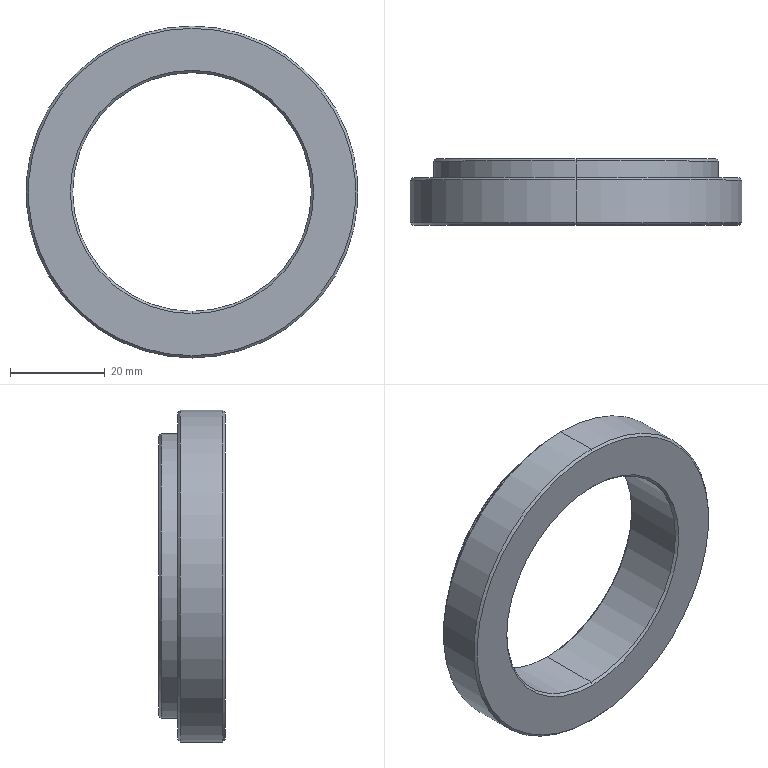Part | STEP file | 10-07 top ring | 1 solid | 19 faces | box 70 x 14 x 70 mm | volume 21857 mm3 | cone 10 | cylinder 6 | plane 3 | commonest cylinder face diameters 50.3 x2 60 x2 70 x2
STEP:
#1=CARTESIAN_POINT('',(0.,3.5,-25.15));
#2=VERTEX_POINT('',#1);
#3=CARTESIAN_POINT('',(0.,3.5,25.15));
#4=VERTEX_POINT('',#3);
#5=CARTESIAN_POINT('',(0.,3.5,0.));
#6=DIRECTION('',(0.,1.,0.));
#7=DIRECTION('',(0.,0.,1.));
#8=AXIS2_PLACEMENT_3D('',#5,#6,#7);
#9=CIRCLE('',#8,25.15);
#10=EDGE_CURVE('',#2,#4,#9,.T.);
#11=ORIENTED_EDGE('',*,*,#10,.F.);
#12=CARTESIAN_POINT('',(0.,4.,-25.65));
#13=VERTEX_POINT('',#12);
#14=CARTESIAN_POINT('',(0.,3.5,-25.15));
#15=DIRECTION('',(0.,0.7071,-0.7071));
#16=VECTOR('',#15,1000.);
#17=LINE('',#14,#16);
#18=EDGE_CURVE('',#2,#13,#17,.T.);
#19=ORIENTED_EDGE('',*,*,#18,.T.);
#20=CARTESIAN_POINT('',(0.,4.,25.65));
#21=VERTEX_POINT('',#20);
#22=CARTESIAN_POINT('',(0.,4.,0.));
#23=DIRECTION('',(0.,-1.,0.));
#24=DIRECTION('',(0.,0.,1.));
#25=AXIS2_PLACEMENT_3D('',#22,#23,#24);
#26=CIRCLE('',#25,25.65);
#27=EDGE_CURVE('',#21,#13,#26,.T.);
#28=ORIENTED_EDGE('',*,*,#27,.F.);
#29=CARTESIAN_POINT('',(0.,3.5,25.15));
#30=DIRECTION('',(0.,0.7071,0.7071));
#31=VECTOR('',#30,1000.);
#32=LINE('',#29,#31);
#33=EDGE_CURVE('',#4,#21,#32,.T.);
#34=ORIENTED_EDGE('',*,*,#33,.F.);
#35=EDGE_LOOP('',(#11,#19,#28,#34));
#36=FACE_OUTER_BOUND('',#35,.T.);
#37=CARTESIAN_POINT('',(0.,3.5,0.));
#38=DIRECTION('',(0.,1.,0.));
#39=DIRECTION('',(0.,0.,1.));
#40=AXIS2_PLACEMENT_3D('',#37,#38,#39);
#41=CONICAL_SURFACE('',#40,25.15,0.7854);
#42=ADVANCED_FACE('',(#36),#41,.F.);
#43=CARTESIAN_POINT('',(0.,4.,29.5));
#44=VERTEX_POINT('',#43);
#45=CARTESIAN_POINT('',(0.,4.,-29.5));
#46=VERTEX_POINT('',#45);
#47=CARTESIAN_POINT('',(0.,4.,0.));
#48=DIRECTION('',(0.,1.,0.));
#49=DIRECTION('',(0.,0.,1.));
#50=AXIS2_PLACEMENT_3D('',#47,#48,#49);
#51=CIRCLE('',#50,29.5);
#52=EDGE_CURVE('',#44,#46,#51,.T.);
#53=ORIENTED_EDGE('',*,*,#52,.F.);
#54=CARTESIAN_POINT('',(0.,3.5,30.));
#55=VERTEX_POINT('',#54);
#56=CARTESIAN_POINT('',(0.,4.,29.5));
#57=DIRECTION('',(0.,-0.7071,0.7071));
#58=VECTOR('',#57,1000.);
#59=LINE('',#56,#58);
#60=EDGE_CURVE('',#44,#55,#59,.T.);
#61=ORIENTED_EDGE('',*,*,#60,.T.);
#62=CARTESIAN_POINT('',(0.,3.5,-30.));
#63=VERTEX_POINT('',#62);
#64=CARTESIAN_POINT('',(0.,3.5,0.));
#65=DIRECTION('',(0.,-1.,0.));
#66=DIRECTION('',(0.,0.,1.));
#67=AXIS2_PLACEMENT_3D('',#64,#65,#66);
#68=CIRCLE('',#67,30.);
#69=EDGE_CURVE('',#63,#55,#68,.T.);
#70=ORIENTED_EDGE('',*,*,#69,.F.);
#71=CARTESIAN_POINT('',(0.,4.,-29.5));
#72=DIRECTION('',(0.,-0.7071,-0.7071));
#73=VECTOR('',#72,1000.);
#74=LINE('',#71,#73);
#75=EDGE_CURVE('',#46,#63,#74,.T.);
#76=ORIENTED_EDGE('',*,*,#75,.F.);
#77=EDGE_LOOP('',(#53,#61,#70,#76));
#78=FACE_OUTER_BOUND('',#77,.T.);
#79=CARTESIAN_POINT('',(0.,4.,0.));
#80=DIRECTION('',(0.,-1.,0.));
#81=DIRECTION('',(0.,0.,-1.));
#82=AXIS2_PLACEMENT_3D('',#79,#80,#81);
#83=CONICAL_SURFACE('',#82,29.5,0.7854);
#84=ADVANCED_FACE('',(#78),#83,.T.);
#85=CARTESIAN_POINT('',(0.,-9.5,25.15));
#86=VERTEX_POINT('',#85);
#87=CARTESIAN_POINT('',(0.,-9.5,-25.15));
#88=VERTEX_POINT('',#87);
#89=CARTESIAN_POINT('',(0.,-9.5,0.));
#90=DIRECTION('',(0.,-1.,0.));
#91=DIRECTION('',(0.,0.,-1.));
#92=AXIS2_PLACEMENT_3D('',#89,#90,#91);
#93=CIRCLE('',#92,25.15);
#94=EDGE_CURVE('',#86,#88,#93,.T.);
#95=ORIENTED_EDGE('',*,*,#94,.F.);
#96=CARTESIAN_POINT('',(0.,-10.,25.65));
#97=VERTEX_POINT('',#96);
#98=CARTESIAN_POINT('',(0.,-9.5,25.15));
#99=DIRECTION('',(0.,-0.7071,0.7071));
#100=VECTOR('',#99,1000.);
#101=LINE('',#98,#100);
#102=EDGE_CURVE('',#86,#97,#101,.T.);
#103=ORIENTED_EDGE('',*,*,#102,.T.);
#104=CARTESIAN_POINT('',(0.,-10.,-25.65));
#105=VERTEX_POINT('',#104);
#106=CARTESIAN_POINT('',(0.,-10.,0.));
#107=DIRECTION('',(0.,1.,0.));
#108=DIRECTION('',(0.,0.,-1.));
#109=AXIS2_PLACEMENT_3D('',#106,#107,#108);
#110=CIRCLE('',#109,25.65);
#111=EDGE_CURVE('',#105,#97,#110,.T.);
#112=ORIENTED_EDGE('',*,*,#111,.F.);
#113=CARTESIAN_POINT('',(0.,-9.5,-25.15));
#114=DIRECTION('',(0.,-0.7071,-0.7071));
#115=VECTOR('',#114,1000.);
#116=LINE('',#113,#115);
#117=EDGE_CURVE('',#88,#105,#116,.T.);
#118=ORIENTED_EDGE('',*,*,#117,.F.);
#119=EDGE_LOOP('',(#95,#103,#112,#118));
#120=FACE_OUTER_BOUND('',#119,.T.);
#121=CARTESIAN_POINT('',(0.,-9.5,0.));
#122=DIRECTION('',(0.,-1.,0.));
#123=DIRECTION('',(0.,0.,-1.));
#124=AXIS2_PLACEMENT_3D('',#121,#122,#123);
#125=CONICAL_SURFACE('',#124,25.15,0.7854);
#126=ADVANCED_FACE('',(#120),#125,.F.);
#127=CARTESIAN_POINT('',(0.,-10.,-34.5));
#128=VERTEX_POINT('',#127);
#129=CARTESIAN_POINT('',(0.,-10.,34.5));
#130=VERTEX_POINT('',#129);
#131=CARTESIAN_POINT('',(0.,-10.,0.));
#132=DIRECTION('',(0.,-1.,0.));
#133=DIRECTION('',(0.,0.,-1.));
#134=AXIS2_PLACEMENT_3D('',#131,#132,#133);
#135=CIRCLE('',#134,34.5);
#136=EDGE_CURVE('',#128,#130,#135,.T.);
#137=ORIENTED_EDGE('',*,*,#136,.F.);
#138=CARTESIAN_POINT('',(0.,-9.5,-35.));
#139=VERTEX_POINT('',#138);
#140=CARTESIAN_POINT('',(0.,-10.,-34.5));
#141=DIRECTION('',(0.,0.7071,-0.7071));
#142=VECTOR('',#141,1000.);
#143=LINE('',#140,#142);
#144=EDGE_CURVE('',#128,#139,#143,.T.);
#145=ORIENTED_EDGE('',*,*,#144,.T.);
#146=CARTESIAN_POINT('',(0.,-9.5,35.));
#147=VERTEX_POINT('',#146);
#148=CARTESIAN_POINT('',(0.,-9.5,0.));
#149=DIRECTION('',(0.,1.,0.));
#150=DIRECTION('',(0.,0.,-1.));
#151=AXIS2_PLACEMENT_3D('',#148,#149,#150);
#152=CIRCLE('',#151,35.);
#153=EDGE_CURVE('',#147,#139,#152,.T.);
#154=ORIENTED_EDGE('',*,*,#153,.F.);
#155=CARTESIAN_POINT('',(0.,-10.,34.5));
#156=DIRECTION('',(0.,0.7071,0.7071));
#157=VECTOR('',#156,1000.);
#158=LINE('',#155,#157);
#159=EDGE_CURVE('',#130,#147,#158,.T.);
#160=ORIENTED_EDGE('',*,*,#159,.F.);
#161=EDGE_LOOP('',(#137,#145,#154,#160));
#162=FACE_OUTER_BOUND('',#161,.T.);
#163=CARTESIAN_POINT('',(0.,-10.,0.));
#164=DIRECTION('',(0.,1.,0.));
#165=DIRECTION('',(0.,0.,1.));
#166=AXIS2_PLACEMENT_3D('',#163,#164,#165);
#167=CONICAL_SURFACE('',#166,34.5,0.7854);
#168=ADVANCED_FACE('',(#162),#167,.T.);
#169=CARTESIAN_POINT('',(0.,0.,34.5));
#170=VERTEX_POINT('',#169);
#171=CARTESIAN_POINT('',(0.,0.,-34.5));
#172=VERTEX_POINT('',#171);
#173=CARTESIAN_POINT('',(0.,0.,0.));
#174=DIRECTION('',(0.,1.,0.));
#175=DIRECTION('',(0.,0.,-1.));
#176=AXIS2_PLACEMENT_3D('',#173,#174,#175);
#177=CIRCLE('',#176,34.5);
#178=EDGE_CURVE('',#170,#172,#177,.T.);
#179=ORIENTED_EDGE('',*,*,#178,.F.);
#180=CARTESIAN_POINT('',(0.,-0.5,35.));
#181=VERTEX_POINT('',#180);
#182=CARTESIAN_POINT('',(0.,-0.5,35.));
#183=DIRECTION('',(0.,-0.7071,0.7071));
#184=VECTOR('',#183,1000.);
#185=LINE('',#182,#184);
#186=EDGE_CURVE('',#170,#181,#185,.T.);
#187=ORIENTED_EDGE('',*,*,#186,.T.);
#188=CARTESIAN_POINT('',(0.,-0.5,-35.));
#189=VERTEX_POINT('',#188);
#190=CARTESIAN_POINT('',(0.,-0.5,0.));
#191=DIRECTION('',(0.,-1.,0.));
#192=DIRECTION('',(0.,0.,-1.));
#193=AXIS2_PLACEMENT_3D('',#190,#191,#192);
#194=CIRCLE('',#193,35.);
#195=EDGE_CURVE('',#189,#181,#194,.T.);
#196=ORIENTED_EDGE('',*,*,#195,.F.);
#197=CARTESIAN_POINT('',(0.,-0.5,-35.));
#198=DIRECTION('',(0.,-0.7071,-0.7071));
#199=VECTOR('',#198,1000.);
#200=LINE('',#197,#199);
#201=EDGE_CURVE('',#172,#189,#200,.T.);
#202=ORIENTED_EDGE('',*,*,#201,.F.);
#203=EDGE_LOOP('',(#179,#187,#196,#202));
#204=FACE_OUTER_BOUND('',#203,.T.);
#205=CARTESIAN_POINT('',(0.,-0.5,0.));
#206=DIRECTION('',(0.,-1.,0.));
#207=DIRECTION('',(0.,0.,-1.));
#208=AXIS2_PLACEMENT_3D('',#205,#206,#207);
#209=CONICAL_SURFACE('',#208,35.,0.7854);
#210=ADVANCED_FACE('',(#204),#209,.T.);
#211=ORIENTED_EDGE('',*,*,#153,.T.);
#212=CARTESIAN_POINT('',(0.,-10.,-35.));
#213=DIRECTION('',(0.,1.,0.));
#214=VECTOR('',#213,1000.);
#215=LINE('',#212,#214);
#216=EDGE_CURVE('',#139,#189,#215,.T.);
#217=ORIENTED_EDGE('',*,*,#216,.T.);
#218=ORIENTED_EDGE('',*,*,#195,.T.);
#219=CARTESIAN_POINT('',(0.,-10.,35.));
#220=DIRECTION('',(0.,1.,0.));
#221=VECTOR('',#220,1000.);
#222=LINE('',#219,#221);
#223=EDGE_CURVE('',#147,#181,#222,.T.);
#224=ORIENTED_EDGE('',*,*,#223,.F.);
#225=EDGE_LOOP('',(#211,#217,#218,#224));
#226=FACE_OUTER_BOUND('',#225,.T.);
#227=CARTESIAN_POINT('',(0.,-10.,0.));
#228=DIRECTION('',(0.,1.,0.));
#229=DIRECTION('',(0.,0.,1.));
#230=AXIS2_PLACEMENT_3D('',#227,#228,#229);
#231=CYLINDRICAL_SURFACE('',#230,35.);
#232=ADVANCED_FACE('',(#226),#231,.T.);
#233=ORIENTED_EDGE('',*,*,#10,.T.);
#234=CARTESIAN_POINT('',(0.,4.,25.15));
#235=DIRECTION('',(0.,-1.,0.));
#236=VECTOR('',#235,1000.);
#237=LINE('',#234,#236);
#238=EDGE_CURVE('',#4,#86,#237,.T.);
#239=ORIENTED_EDGE('',*,*,#238,.T.);
#240=ORIENTED_EDGE('',*,*,#94,.T.);
#241=CARTESIAN_POINT('',(0.,4.,-25.15));
#242=DIRECTION('',(0.,-1.,0.));
#243=VECTOR('',#242,1000.);
#244=LINE('',#241,#243);
#245=EDGE_CURVE('',#2,#88,#244,.T.);
#246=ORIENTED_EDGE('',*,*,#245,.F.);
#247=EDGE_LOOP('',(#233,#239,#240,#246));
#248=FACE_OUTER_BOUND('',#247,.T.);
#249=CARTESIAN_POINT('',(0.,4.,0.));
#250=DIRECTION('',(0.,-1.,0.));
#251=DIRECTION('',(0.,0.,-1.));
#252=AXIS2_PLACEMENT_3D('',#249,#250,#251);
#253=CYLINDRICAL_SURFACE('',#252,25.15);
#254=ADVANCED_FACE('',(#248),#253,.F.);
#255=ORIENTED_EDGE('',*,*,#69,.T.);
#256=CARTESIAN_POINT('',(0.,0.,30.));
#257=VERTEX_POINT('',#256);
#258=CARTESIAN_POINT('',(0.,4.,30.));
#259=DIRECTION('',(0.,-1.,0.));
#260=VECTOR('',#259,1000.);
#261=LINE('',#258,#260);
#262=EDGE_CURVE('',#55,#257,#261,.T.);
#263=ORIENTED_EDGE('',*,*,#262,.T.);
#264=CARTESIAN_POINT('',(0.,0.,-30.));
#265=VERTEX_POINT('',#264);
#266=CARTESIAN_POINT('',(0.,0.,0.));
#267=DIRECTION('',(0.,-1.,0.));
#268=DIRECTION('',(0.,0.,-1.));
#269=AXIS2_PLACEMENT_3D('',#266,#267,#268);
#270=CIRCLE('',#269,30.);
#271=EDGE_CURVE('',#265,#257,#270,.T.);
#272=ORIENTED_EDGE('',*,*,#271,.F.);
#273=CARTESIAN_POINT('',(0.,4.,-30.));
#274=DIRECTION('',(0.,-1.,0.));
#275=VECTOR('',#274,1000.);
#276=LINE('',#273,#275);
#277=EDGE_CURVE('',#63,#265,#276,.T.);
#278=ORIENTED_EDGE('',*,*,#277,.F.);
#279=EDGE_LOOP('',(#255,#263,#272,#278));
#280=FACE_OUTER_BOUND('',#279,.T.);
#281=CARTESIAN_POINT('',(0.,4.,0.));
#282=DIRECTION('',(0.,-1.,0.));
#283=DIRECTION('',(0.,0.,-1.));
#284=AXIS2_PLACEMENT_3D('',#281,#282,#283);
#285=CYLINDRICAL_SURFACE('',#284,30.);
#286=ADVANCED_FACE('',(#280),#285,.T.);
#287=CARTESIAN_POINT('',(0.,4.,0.));
#288=DIRECTION('',(0.,1.,0.));
#289=DIRECTION('',(0.,0.,1.));
#290=AXIS2_PLACEMENT_3D('',#287,#288,#289);
#291=CIRCLE('',#290,29.5);
#292=EDGE_CURVE('',#46,#44,#291,.T.);
#293=ORIENTED_EDGE('',*,*,#292,.T.);
#294=ORIENTED_EDGE('',*,*,#52,.T.);
#295=EDGE_LOOP('',(#293,#294));
#296=FACE_OUTER_BOUND('',#295,.T.);
#297=ORIENTED_EDGE('',*,*,#27,.T.);
#298=CARTESIAN_POINT('',(0.,4.,0.));
#299=DIRECTION('',(0.,-1.,0.));
#300=DIRECTION('',(0.,0.,1.));
#301=AXIS2_PLACEMENT_3D('',#298,#299,#300);
#302=CIRCLE('',#301,25.65);
#303=EDGE_CURVE('',#13,#21,#302,.T.);
#304=ORIENTED_EDGE('',*,*,#303,.T.);
#305=EDGE_LOOP('',(#297,#304));
#306=FACE_BOUND('',#305,.T.);
#307=CARTESIAN_POINT('',(0.,4.,0.));
#308=DIRECTION('',(0.,1.,0.));
#309=DIRECTION('',(0.,0.,1.));
#310=AXIS2_PLACEMENT_3D('',#307,#308,#309);
#311=PLANE('',#310);
#312=ADVANCED_FACE('',(#296,#306),#311,.T.);
#313=ORIENTED_EDGE('',*,*,#262,.F.);
#314=CARTESIAN_POINT('',(0.,3.5,0.));
#315=DIRECTION('',(0.,-1.,0.));
#316=DIRECTION('',(0.,0.,1.));
#317=AXIS2_PLACEMENT_3D('',#314,#315,#316);
#318=CIRCLE('',#317,30.);
#319=EDGE_CURVE('',#55,#63,#318,.T.);
#320=ORIENTED_EDGE('',*,*,#319,.T.);
#321=ORIENTED_EDGE('',*,*,#277,.T.);
#322=CARTESIAN_POINT('',(0.,0.,0.));
#323=DIRECTION('',(0.,-1.,0.));
#324=DIRECTION('',(0.,0.,-1.));
#325=AXIS2_PLACEMENT_3D('',#322,#323,#324);
#326=CIRCLE('',#325,30.);
#327=EDGE_CURVE('',#257,#265,#326,.T.);
#328=ORIENTED_EDGE('',*,*,#327,.F.);
#329=EDGE_LOOP('',(#313,#320,#321,#328));
#330=FACE_OUTER_BOUND('',#329,.T.);
#331=CARTESIAN_POINT('',(0.,4.,0.));
#332=DIRECTION('',(0.,-1.,0.));
#333=DIRECTION('',(0.,0.,-1.));
#334=AXIS2_PLACEMENT_3D('',#331,#332,#333);
#335=CYLINDRICAL_SURFACE('',#334,30.);
#336=ADVANCED_FACE('',(#330),#335,.T.);
#337=ORIENTED_EDGE('',*,*,#238,.F.);
#338=CARTESIAN_POINT('',(0.,3.5,0.));
#339=DIRECTION('',(0.,1.,0.));
#340=DIRECTION('',(0.,0.,1.));
#341=AXIS2_PLACEMENT_3D('',#338,#339,#340);
#342=CIRCLE('',#341,25.15);
#343=EDGE_CURVE('',#4,#2,#342,.T.);
#344=ORIENTED_EDGE('',*,*,#343,.T.);
#345=ORIENTED_EDGE('',*,*,#245,.T.);
#346=CARTESIAN_POINT('',(0.,-9.5,0.));
#347=DIRECTION('',(0.,-1.,0.));
#348=DIRECTION('',(0.,0.,-1.));
#349=AXIS2_PLACEMENT_3D('',#346,#347,#348);
#350=CIRCLE('',#349,25.15);
#351=EDGE_CURVE('',#88,#86,#350,.T.);
#352=ORIENTED_EDGE('',*,*,#351,.T.);
#353=EDGE_LOOP('',(#337,#344,#345,#352));
#354=FACE_OUTER_BOUND('',#353,.T.);
#355=CARTESIAN_POINT('',(0.,4.,0.));
#356=DIRECTION('',(0.,-1.,0.));
#357=DIRECTION('',(0.,0.,-1.));
#358=AXIS2_PLACEMENT_3D('',#355,#356,#357);
#359=CYLINDRICAL_SURFACE('',#358,25.15);
#360=ADVANCED_FACE('',(#354),#359,.F.);
#361=CARTESIAN_POINT('',(0.,0.,0.));
#362=DIRECTION('',(0.,1.,0.));
#363=DIRECTION('',(0.,0.,-1.));
#364=AXIS2_PLACEMENT_3D('',#361,#362,#363);
#365=CIRCLE('',#364,34.5);
#366=EDGE_CURVE('',#172,#170,#365,.T.);
#367=ORIENTED_EDGE('',*,*,#366,.T.);
#368=ORIENTED_EDGE('',*,*,#178,.T.);
#369=EDGE_LOOP('',(#367,#368));
#370=FACE_OUTER_BOUND('',#369,.T.);
#371=ORIENTED_EDGE('',*,*,#271,.T.);
#372=ORIENTED_EDGE('',*,*,#327,.T.);
#373=EDGE_LOOP('',(#371,#372));
#374=FACE_BOUND('',#373,.T.);
#375=CARTESIAN_POINT('',(0.,0.,0.));
#376=DIRECTION('',(0.,-1.,0.));
#377=DIRECTION('',(0.,0.,-1.));
#378=AXIS2_PLACEMENT_3D('',#375,#376,#377);
#379=PLANE('',#378);
#380=ADVANCED_FACE('',(#370,#374),#379,.F.);
#381=CARTESIAN_POINT('',(0.,-10.,0.));
#382=DIRECTION('',(0.,-1.,0.));
#383=DIRECTION('',(0.,0.,-1.));
#384=AXIS2_PLACEMENT_3D('',#381,#382,#383);
#385=CIRCLE('',#384,34.5);
#386=EDGE_CURVE('',#130,#128,#385,.T.);
#387=ORIENTED_EDGE('',*,*,#386,.T.);
#388=ORIENTED_EDGE('',*,*,#136,.T.);
#389=EDGE_LOOP('',(#387,#388));
#390=FACE_OUTER_BOUND('',#389,.T.);
#391=ORIENTED_EDGE('',*,*,#111,.T.);
#392=CARTESIAN_POINT('',(0.,-10.,0.));
#393=DIRECTION('',(0.,1.,0.));
#394=DIRECTION('',(0.,0.,-1.));
#395=AXIS2_PLACEMENT_3D('',#392,#393,#394);
#396=CIRCLE('',#395,25.65);
#397=EDGE_CURVE('',#97,#105,#396,.T.);
#398=ORIENTED_EDGE('',*,*,#397,.T.);
#399=EDGE_LOOP('',(#391,#398));
#400=FACE_BOUND('',#399,.T.);
#401=CARTESIAN_POINT('',(0.,-10.,0.));
#402=DIRECTION('',(0.,-1.,0.));
#403=DIRECTION('',(0.,0.,-1.));
#404=AXIS2_PLACEMENT_3D('',#401,#402,#403);
#405=PLANE('',#404);
#406=ADVANCED_FACE('',(#390,#400),#405,.T.);
#407=ORIENTED_EDGE('',*,*,#216,.F.);
#408=CARTESIAN_POINT('',(0.,-9.5,0.));
#409=DIRECTION('',(0.,1.,0.));
#410=DIRECTION('',(0.,0.,-1.));
#411=AXIS2_PLACEMENT_3D('',#408,#409,#410);
#412=CIRCLE('',#411,35.);
#413=EDGE_CURVE('',#139,#147,#412,.T.);
#414=ORIENTED_EDGE('',*,*,#413,.T.);
#415=ORIENTED_EDGE('',*,*,#223,.T.);
#416=CARTESIAN_POINT('',(0.,-0.5,0.));
#417=DIRECTION('',(0.,-1.,0.));
#418=DIRECTION('',(0.,0.,-1.));
#419=AXIS2_PLACEMENT_3D('',#416,#417,#418);
#420=CIRCLE('',#419,35.);
#421=EDGE_CURVE('',#181,#189,#420,.T.);
#422=ORIENTED_EDGE('',*,*,#421,.T.);
#423=EDGE_LOOP('',(#407,#414,#415,#422));
#424=FACE_OUTER_BOUND('',#423,.T.);
#425=CARTESIAN_POINT('',(0.,-10.,0.));
#426=DIRECTION('',(0.,1.,0.));
#427=DIRECTION('',(0.,0.,1.));
#428=AXIS2_PLACEMENT_3D('',#425,#426,#427);
#429=CYLINDRICAL_SURFACE('',#428,35.);
#430=ADVANCED_FACE('',(#424),#429,.T.);
#431=ORIENTED_EDGE('',*,*,#186,.F.);
#432=ORIENTED_EDGE('',*,*,#366,.F.);
#433=ORIENTED_EDGE('',*,*,#201,.T.);
#434=ORIENTED_EDGE('',*,*,#421,.F.);
#435=EDGE_LOOP('',(#431,#432,#433,#434));
#436=FACE_OUTER_BOUND('',#435,.T.);
#437=CARTESIAN_POINT('',(0.,-0.5,0.));
#438=DIRECTION('',(0.,-1.,0.));
#439=DIRECTION('',(0.,0.,-1.));
#440=AXIS2_PLACEMENT_3D('',#437,#438,#439);
#441=CONICAL_SURFACE('',#440,35.,0.7854);
#442=ADVANCED_FACE('',(#436),#441,.T.);
#443=ORIENTED_EDGE('',*,*,#144,.F.);
#444=ORIENTED_EDGE('',*,*,#386,.F.);
#445=ORIENTED_EDGE('',*,*,#159,.T.);
#446=ORIENTED_EDGE('',*,*,#413,.F.);
#447=EDGE_LOOP('',(#443,#444,#445,#446));
#448=FACE_OUTER_BOUND('',#447,.T.);
#449=CARTESIAN_POINT('',(0.,-10.,0.));
#450=DIRECTION('',(0.,1.,0.));
#451=DIRECTION('',(0.,0.,1.));
#452=AXIS2_PLACEMENT_3D('',#449,#450,#451);
#453=CONICAL_SURFACE('',#452,34.5,0.7854);
#454=ADVANCED_FACE('',(#448),#453,.T.);
#455=ORIENTED_EDGE('',*,*,#102,.F.);
#456=ORIENTED_EDGE('',*,*,#351,.F.);
#457=ORIENTED_EDGE('',*,*,#117,.T.);
#458=ORIENTED_EDGE('',*,*,#397,.F.);
#459=EDGE_LOOP('',(#455,#456,#457,#458));
#460=FACE_OUTER_BOUND('',#459,.T.);
#461=CARTESIAN_POINT('',(0.,-9.5,0.));
#462=DIRECTION('',(0.,-1.,0.));
#463=DIRECTION('',(0.,0.,-1.));
#464=AXIS2_PLACEMENT_3D('',#461,#462,#463);
#465=CONICAL_SURFACE('',#464,25.15,0.7854);
#466=ADVANCED_FACE('',(#460),#465,.F.);
#467=ORIENTED_EDGE('',*,*,#60,.F.);
#468=ORIENTED_EDGE('',*,*,#292,.F.);
#469=ORIENTED_EDGE('',*,*,#75,.T.);
#470=ORIENTED_EDGE('',*,*,#319,.F.);
#471=EDGE_LOOP('',(#467,#468,#469,#470));
#472=FACE_OUTER_BOUND('',#471,.T.);
#473=CARTESIAN_POINT('',(0.,4.,0.));
#474=DIRECTION('',(0.,-1.,0.));
#475=DIRECTION('',(0.,0.,-1.));
#476=AXIS2_PLACEMENT_3D('',#473,#474,#475);
#477=CONICAL_SURFACE('',#476,29.5,0.7854);
#478=ADVANCED_FACE('',(#472),#477,.T.);
#479=ORIENTED_EDGE('',*,*,#18,.F.);
#480=ORIENTED_EDGE('',*,*,#343,.F.);
#481=ORIENTED_EDGE('',*,*,#33,.T.);
#482=ORIENTED_EDGE('',*,*,#303,.F.);
#483=EDGE_LOOP('',(#479,#480,#481,#482));
#484=FACE_OUTER_BOUND('',#483,.T.);
#485=CARTESIAN_POINT('',(0.,3.5,0.));
#486=DIRECTION('',(0.,1.,0.));
#487=DIRECTION('',(0.,0.,1.));
#488=AXIS2_PLACEMENT_3D('',#485,#486,#487);
#489=CONICAL_SURFACE('',#488,25.15,0.7854);
#490=ADVANCED_FACE('',(#484),#489,.F.);
#491=CLOSED_SHELL('',(#42,#84,#126,#168,#210,#232,#254,#286,#312,#336,#360,#380,#406,#430,#442,#454,#466,#478,#490));
#492=MANIFOLD_SOLID_BREP('',#491);
#493=CARTESIAN_POINT('',(0.,0.,0.));
#494=DIRECTION('',(0.,0.,1.));
#495=DIRECTION('',(1.,0.,0.));
#496=AXIS2_PLACEMENT_3D('',#493,#494,#495);
#497=(LENGTH_UNIT()NAMED_UNIT(*)SI_UNIT(.MILLI.,.METRE.));
#498=UNCERTAINTY_MEASURE_WITH_UNIT(LENGTH_MEASURE(0.00001),#497,'','');
#499=(NAMED_UNIT(*)PLANE_ANGLE_UNIT()SI_UNIT($,.RADIAN.));
#500=(NAMED_UNIT(*)SI_UNIT($,.STERADIAN.)SOLID_ANGLE_UNIT());
#501=(GEOMETRIC_REPRESENTATION_CONTEXT(3)GLOBAL_UNCERTAINTY_ASSIGNED_CONTEXT((#498))GLOBAL_UNIT_ASSIGNED_CONTEXT((#497,#499,#500))REPRESENTATION_CONTEXT('',''));
#502=ADVANCED_BREP_SHAPE_REPRESENTATION('',(#492,#496),#501);